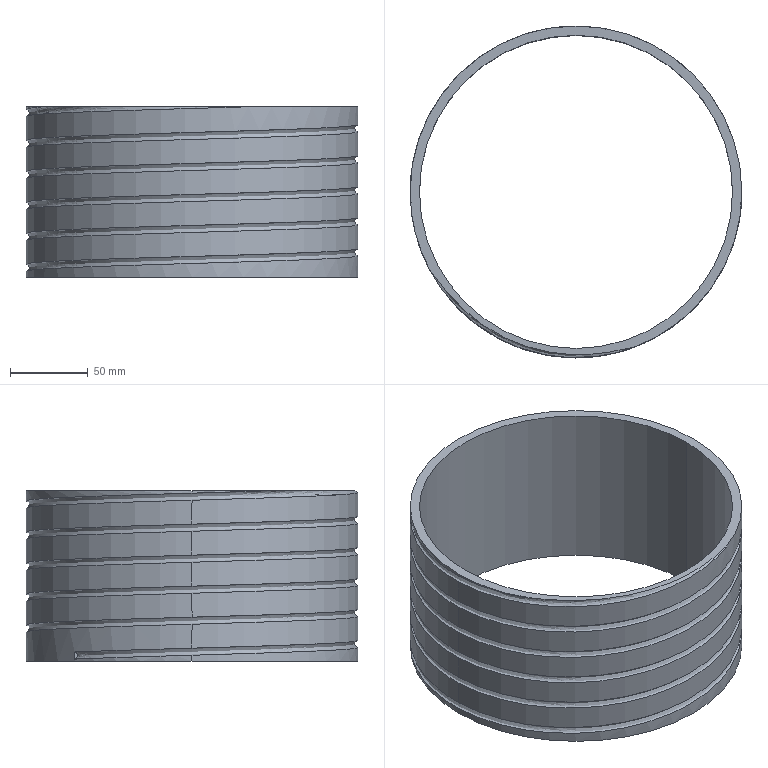Part | SolidWorks | features Extrusion 1, Helix 1, SweepCut 1 | 1 solid | 19 faces | volume 402260 mm3 | cylinder 15 | plane 3 | spline 1 | commonest cylinder face diameters 214 x13 202 x2